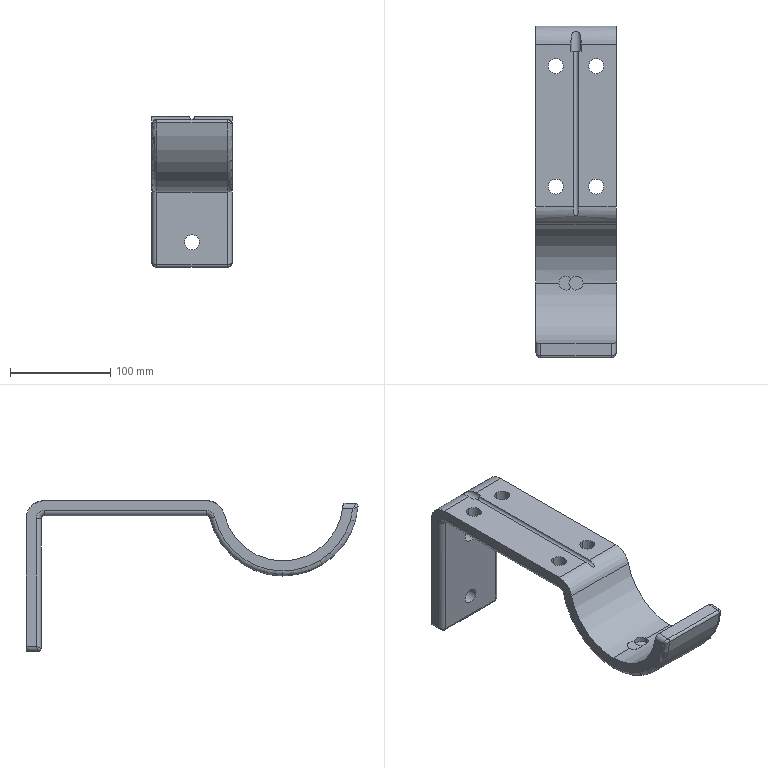Part | STEP file | Input 132 | 1 solid | 60 faces | box 80 x 330.779 x 150 mm | volume 596739 mm3 | cylinder 36 | plane 12 | torus 8 | spline 4 | commonest cylinder face diameters 15 x12 10 x9 14 x4 5 x3 6 x2 36 x2